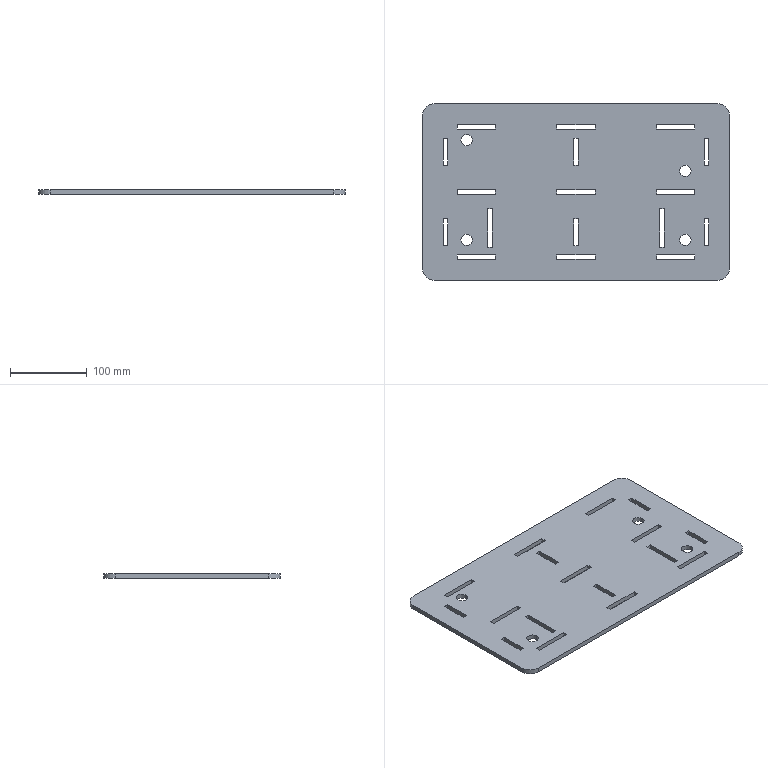Part | SolidWorks | features FlatPattern 1, SMBaseFlange 1, SheetMetal 1 | 1 solid | 86 faces | box 400 x 230 x 6 mm | volume 519240 mm3 | plane 74 | cylinder 12 | commonest cylinder face diameters 15 x8 30 x4